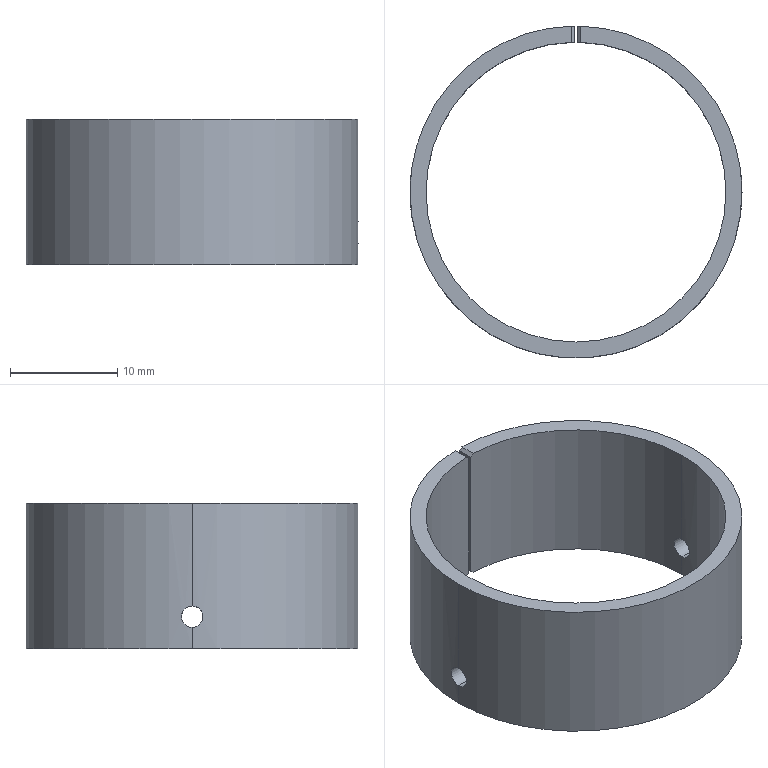Part | STEP file | TQ-DD-1105-THSHIELD1010_デフォルト | 1 solid | 18 faces | box 31 x 30.999 x 13.6 mm | volume 1876 mm3 | cylinder 10 | plane 8 | commonest cylinder face diameters 2 x4 28 x3 31 x3
STEP:
#1=CARTESIAN_POINT('',(-0.4352,15.494,0.));
#2=VERTEX_POINT('',#1);
#3=CARTESIAN_POINT('',(-15.5,0.,0.));
#4=VERTEX_POINT('',#3);
#5=CARTESIAN_POINT('',(0.,0.,0.));
#6=DIRECTION('',(0.,0.,1.));
#7=DIRECTION('',(1.,0.,0.));
#8=AXIS2_PLACEMENT_3D('',#5,#6,#7);
#9=CIRCLE('',#8,15.5);
#10=EDGE_CURVE('',#2,#4,#9,.T.);
#11=ORIENTED_EDGE('',*,*,#10,.T.);
#12=CARTESIAN_POINT('',(-15.5,0.,2.));
#13=VERTEX_POINT('',#12);
#14=CARTESIAN_POINT('',(-15.5,0.,6.8));
#15=DIRECTION('',(0.,0.,1.));
#16=VECTOR('',#15,1000.);
#17=LINE('',#14,#16);
#18=EDGE_CURVE('',#4,#13,#17,.T.);
#19=ORIENTED_EDGE('',*,*,#18,.T.);
#20=CARTESIAN_POINT('',(-15.5,0.,4.));
#21=VERTEX_POINT('',#20);
#22=CARTESIAN_POINT('',(-15.5,0.,2.));
#23=CARTESIAN_POINT('',(-15.5,0.1305,2.));
#24=CARTESIAN_POINT('',(-15.498,0.2615,2.026));
#25=CARTESIAN_POINT('',(-15.492,0.5036,2.126));
#26=CARTESIAN_POINT('',(-15.488,0.6138,2.2));
#27=CARTESIAN_POINT('',(-15.48,0.8004,2.386));
#28=CARTESIAN_POINT('',(-15.475,0.8738,2.496));
#29=CARTESIAN_POINT('',(-15.469,0.9741,2.739));
#30=CARTESIAN_POINT('',(-15.468,1.,2.869));
#31=CARTESIAN_POINT('',(-15.468,0.9999,3.133));
#32=CARTESIAN_POINT('',(-15.469,0.9738,3.263));
#33=CARTESIAN_POINT('',(-15.475,0.8732,3.505));
#34=CARTESIAN_POINT('',(-15.48,0.7989,3.615));
#35=CARTESIAN_POINT('',(-15.488,0.6143,3.8));
#36=CARTESIAN_POINT('',(-15.492,0.5027,3.874));
#37=CARTESIAN_POINT('',(-15.498,0.2621,3.974));
#38=CARTESIAN_POINT('',(-15.5,0.1305,4.));
#39=CARTESIAN_POINT('',(-15.5,0.,4.));
#40=B_SPLINE_CURVE_WITH_KNOTS('',3,(#22,#23,#24,#25,#26,#27,#28,#29,#30,#31,#32,#33,#34,#35,#36,#37,#38,#39),.UNSPECIFIED.,.F.,.F.,(4,2,2,2,2,2,2,2,4),(0.001564,0.001955,0.002346,0.002736,0.003127,0.003518,0.003909,0.0043,0.004691),.UNSPECIFIED.);
#41=EDGE_CURVE('',#13,#21,#40,.T.);
#42=ORIENTED_EDGE('',*,*,#41,.T.);
#43=CARTESIAN_POINT('',(-15.5,0.,13.6));
#44=VERTEX_POINT('',#43);
#45=CARTESIAN_POINT('',(-15.5,0.,6.8));
#46=DIRECTION('',(0.,0.,1.));
#47=VECTOR('',#46,1000.);
#48=LINE('',#45,#47);
#49=EDGE_CURVE('',#21,#44,#48,.T.);
#50=ORIENTED_EDGE('',*,*,#49,.T.);
#51=CARTESIAN_POINT('',(-0.4352,15.494,13.6));
#52=VERTEX_POINT('',#51);
#53=CARTESIAN_POINT('',(0.,0.,13.6));
#54=DIRECTION('',(0.,0.,-1.));
#55=DIRECTION('',(1.,0.,0.));
#56=AXIS2_PLACEMENT_3D('',#53,#54,#55);
#57=CIRCLE('',#56,15.5);
#58=EDGE_CURVE('',#44,#52,#57,.T.);
#59=ORIENTED_EDGE('',*,*,#58,.T.);
#60=CARTESIAN_POINT('',(-0.1353,15.499,13.3));
#61=VERTEX_POINT('',#60);
#62=CARTESIAN_POINT('',(-0.1353,15.499,13.3));
#63=CARTESIAN_POINT('',(-0.2353,15.499,13.4));
#64=CARTESIAN_POINT('',(-0.3353,15.497,13.5));
#65=CARTESIAN_POINT('',(-0.4352,15.494,13.6));
#66=(BOUNDED_CURVE()B_SPLINE_CURVE(3,(#62,#63,#64,#65),.UNSPECIFIED.,.F.,.F.)B_SPLINE_CURVE_WITH_KNOTS((4,4),(4.712,4.732),.UNSPECIFIED.)CURVE()GEOMETRIC_REPRESENTATION_ITEM()RATIONAL_B_SPLINE_CURVE((1.,1.,1.,1.))REPRESENTATION_ITEM(''));
#67=EDGE_CURVE('',#61,#52,#66,.T.);
#68=ORIENTED_EDGE('',*,*,#67,.F.);
#69=CARTESIAN_POINT('',(-0.1353,15.499,0.3));
#70=VERTEX_POINT('',#69);
#71=CARTESIAN_POINT('',(-0.1353,15.499,6.8));
#72=DIRECTION('',(0.,0.,-1.));
#73=VECTOR('',#72,1000.);
#74=LINE('',#71,#73);
#75=EDGE_CURVE('',#61,#70,#74,.T.);
#76=ORIENTED_EDGE('',*,*,#75,.T.);
#77=CARTESIAN_POINT('',(-0.1353,15.499,0.3));
#78=CARTESIAN_POINT('',(-0.2353,15.499,0.2));
#79=CARTESIAN_POINT('',(-0.3353,15.497,0.09999));
#80=CARTESIAN_POINT('',(-0.4352,15.494,0.));
#81=(BOUNDED_CURVE()B_SPLINE_CURVE(3,(#77,#78,#79,#80),.UNSPECIFIED.,.F.,.F.)B_SPLINE_CURVE_WITH_KNOTS((4,4),(1.571,1.59),.UNSPECIFIED.)CURVE()GEOMETRIC_REPRESENTATION_ITEM()RATIONAL_B_SPLINE_CURVE((1.,1.,1.,1.))REPRESENTATION_ITEM(''));
#82=EDGE_CURVE('',#70,#2,#81,.T.);
#83=ORIENTED_EDGE('',*,*,#82,.T.);
#84=EDGE_LOOP('',(#11,#19,#42,#50,#59,#68,#76,#83));
#85=FACE_OUTER_BOUND('',#84,.T.);
#86=CARTESIAN_POINT('',(0.,0.,6.8));
#87=DIRECTION('',(0.,0.,1.));
#88=DIRECTION('',(1.,0.,0.));
#89=AXIS2_PLACEMENT_3D('',#86,#87,#88);
#90=CYLINDRICAL_SURFACE('',#89,15.5);
#91=ADVANCED_FACE('',(#85),#90,.T.);
#92=ORIENTED_EDGE('',*,*,#18,.F.);
#93=CARTESIAN_POINT('',(15.5,0.,0.));
#94=VERTEX_POINT('',#93);
#95=CARTESIAN_POINT('',(0.,0.,0.));
#96=DIRECTION('',(0.,0.,1.));
#97=DIRECTION('',(1.,0.,0.));
#98=AXIS2_PLACEMENT_3D('',#95,#96,#97);
#99=CIRCLE('',#98,15.5);
#100=EDGE_CURVE('',#4,#94,#99,.T.);
#101=ORIENTED_EDGE('',*,*,#100,.T.);
#102=CARTESIAN_POINT('',(15.5,0.,2.));
#103=VERTEX_POINT('',#102);
#104=CARTESIAN_POINT('',(15.5,0.,6.8));
#105=DIRECTION('',(0.,0.,1.));
#106=VECTOR('',#105,1000.);
#107=LINE('',#104,#106);
#108=EDGE_CURVE('',#94,#103,#107,.T.);
#109=ORIENTED_EDGE('',*,*,#108,.T.);
#110=CARTESIAN_POINT('',(15.5,0.,4.));
#111=VERTEX_POINT('',#110);
#112=CARTESIAN_POINT('',(15.5,0.,2.));
#113=CARTESIAN_POINT('',(15.5,-0.1305,2.));
#114=CARTESIAN_POINT('',(15.498,-0.2615,2.026));
#115=CARTESIAN_POINT('',(15.492,-0.5036,2.126));
#116=CARTESIAN_POINT('',(15.488,-0.6137,2.2));
#117=CARTESIAN_POINT('',(15.48,-0.8004,2.386));
#118=CARTESIAN_POINT('',(15.475,-0.8738,2.496));
#119=CARTESIAN_POINT('',(15.469,-0.9741,2.739));
#120=CARTESIAN_POINT('',(15.468,-1.,2.869));
#121=CARTESIAN_POINT('',(15.468,-0.9999,3.133));
#122=CARTESIAN_POINT('',(15.469,-0.9738,3.263));
#123=CARTESIAN_POINT('',(15.475,-0.8732,3.505));
#124=CARTESIAN_POINT('',(15.48,-0.7989,3.615));
#125=CARTESIAN_POINT('',(15.488,-0.6143,3.8));
#126=CARTESIAN_POINT('',(15.492,-0.5027,3.874));
#127=CARTESIAN_POINT('',(15.498,-0.2621,3.974));
#128=CARTESIAN_POINT('',(15.5,-0.1305,4.));
#129=CARTESIAN_POINT('',(15.5,0.,4.));
#130=B_SPLINE_CURVE_WITH_KNOTS('',3,(#112,#113,#114,#115,#116,#117,#118,#119,#120,#121,#122,#123,#124,#125,#126,#127,#128,#129),.UNSPECIFIED.,.F.,.F.,(4,2,2,2,2,2,2,2,4),(0.004691,0.005081,0.005472,0.005863,0.006254,0.006645,0.007036,0.007426,0.007817),.UNSPECIFIED.);
#131=EDGE_CURVE('',#103,#111,#130,.T.);
#132=ORIENTED_EDGE('',*,*,#131,.T.);
#133=CARTESIAN_POINT('',(15.5,0.,13.6));
#134=VERTEX_POINT('',#133);
#135=CARTESIAN_POINT('',(15.5,0.,6.8));
#136=DIRECTION('',(0.,0.,1.));
#137=VECTOR('',#136,1000.);
#138=LINE('',#135,#137);
#139=EDGE_CURVE('',#111,#134,#138,.T.);
#140=ORIENTED_EDGE('',*,*,#139,.T.);
#141=CARTESIAN_POINT('',(0.,0.,13.6));
#142=DIRECTION('',(0.,0.,-1.));
#143=DIRECTION('',(1.,0.,0.));
#144=AXIS2_PLACEMENT_3D('',#141,#142,#143);
#145=CIRCLE('',#144,15.5);
#146=EDGE_CURVE('',#134,#44,#145,.T.);
#147=ORIENTED_EDGE('',*,*,#146,.T.);
#148=ORIENTED_EDGE('',*,*,#49,.F.);
#149=CARTESIAN_POINT('',(-15.5,0.,4.));
#150=CARTESIAN_POINT('',(-15.5,-0.1305,4.));
#151=CARTESIAN_POINT('',(-15.498,-0.2615,3.974));
#152=CARTESIAN_POINT('',(-15.492,-0.5036,3.874));
#153=CARTESIAN_POINT('',(-15.488,-0.6137,3.8));
#154=CARTESIAN_POINT('',(-15.48,-0.8004,3.614));
#155=CARTESIAN_POINT('',(-15.475,-0.8738,3.504));
#156=CARTESIAN_POINT('',(-15.469,-0.9741,3.261));
#157=CARTESIAN_POINT('',(-15.468,-1.,3.131));
#158=CARTESIAN_POINT('',(-15.468,-0.9999,2.867));
#159=CARTESIAN_POINT('',(-15.469,-0.9738,2.737));
#160=CARTESIAN_POINT('',(-15.475,-0.8732,2.495));
#161=CARTESIAN_POINT('',(-15.48,-0.7989,2.385));
#162=CARTESIAN_POINT('',(-15.488,-0.6143,2.2));
#163=CARTESIAN_POINT('',(-15.492,-0.5027,2.126));
#164=CARTESIAN_POINT('',(-15.498,-0.2621,2.026));
#165=CARTESIAN_POINT('',(-15.5,-0.1305,2.));
#166=CARTESIAN_POINT('',(-15.5,0.,2.));
#167=B_SPLINE_CURVE_WITH_KNOTS('',3,(#149,#150,#151,#152,#153,#154,#155,#156,#157,#158,#159,#160,#161,#162,#163,#164,#165,#166),.UNSPECIFIED.,.F.,.F.,(4,2,2,2,2,2,2,2,4),(0.004691,0.005081,0.005472,0.005863,0.006254,0.006645,0.007036,0.007426,0.007817),.UNSPECIFIED.);
#168=EDGE_CURVE('',#21,#13,#167,.T.);
#169=ORIENTED_EDGE('',*,*,#168,.T.);
#170=EDGE_LOOP('',(#92,#101,#109,#132,#140,#147,#148,#169));
#171=FACE_OUTER_BOUND('',#170,.T.);
#172=CARTESIAN_POINT('',(0.,0.,6.8));
#173=DIRECTION('',(0.,0.,1.));
#174=DIRECTION('',(1.,0.,0.));
#175=AXIS2_PLACEMENT_3D('',#172,#173,#174);
#176=CYLINDRICAL_SURFACE('',#175,15.5);
#177=ADVANCED_FACE('',(#171),#176,.T.);
#178=CARTESIAN_POINT('',(14.,0.,4.));
#179=VERTEX_POINT('',#178);
#180=CARTESIAN_POINT('',(14.,0.,2.));
#181=VERTEX_POINT('',#180);
#182=CARTESIAN_POINT('',(14.,0.,4.));
#183=CARTESIAN_POINT('',(14.,-0.1305,4.));
#184=CARTESIAN_POINT('',(13.998,-0.2615,3.974));
#185=CARTESIAN_POINT('',(13.991,-0.5037,3.874));
#186=CARTESIAN_POINT('',(13.987,-0.6138,3.8));
#187=CARTESIAN_POINT('',(13.977,-0.8005,3.614));
#188=CARTESIAN_POINT('',(13.973,-0.8738,3.504));
#189=CARTESIAN_POINT('',(13.966,-0.9741,3.261));
#190=CARTESIAN_POINT('',(13.964,-1.,3.131));
#191=CARTESIAN_POINT('',(13.964,-0.9999,2.867));
#192=CARTESIAN_POINT('',(13.966,-0.9738,2.737));
#193=CARTESIAN_POINT('',(13.973,-0.8732,2.495));
#194=CARTESIAN_POINT('',(13.977,-0.7989,2.385));
#195=CARTESIAN_POINT('',(13.987,-0.6143,2.2));
#196=CARTESIAN_POINT('',(13.991,-0.5028,2.126));
#197=CARTESIAN_POINT('',(13.998,-0.2621,2.026));
#198=CARTESIAN_POINT('',(14.,-0.1305,2.));
#199=CARTESIAN_POINT('',(14.,0.,2.));
#200=B_SPLINE_CURVE_WITH_KNOTS('',3,(#182,#183,#184,#185,#186,#187,#188,#189,#190,#191,#192,#193,#194,#195,#196,#197,#198,#199),.UNSPECIFIED.,.F.,.F.,(4,2,2,2,2,2,2,2,4),(0.004691,0.005082,0.005473,0.005863,0.006254,0.006645,0.007036,0.007427,0.007818),.UNSPECIFIED.);
#201=EDGE_CURVE('',#179,#181,#200,.T.);
#202=ORIENTED_EDGE('',*,*,#201,.F.);
#203=CARTESIAN_POINT('',(0.,0.,4.));
#204=DIRECTION('',(1.,0.,0.));
#205=VECTOR('',#204,1000.);
#206=LINE('',#203,#205);
#207=EDGE_CURVE('',#179,#111,#206,.T.);
#208=ORIENTED_EDGE('',*,*,#207,.T.);
#209=ORIENTED_EDGE('',*,*,#131,.F.);
#210=CARTESIAN_POINT('',(0.,0.,2.));
#211=DIRECTION('',(1.,0.,0.));
#212=VECTOR('',#211,1000.);
#213=LINE('',#210,#212);
#214=EDGE_CURVE('',#181,#103,#213,.T.);
#215=ORIENTED_EDGE('',*,*,#214,.F.);
#216=EDGE_LOOP('',(#202,#208,#209,#215));
#217=FACE_OUTER_BOUND('',#216,.T.);
#218=CARTESIAN_POINT('',(0.,0.,3.));
#219=DIRECTION('',(1.,0.,0.));
#220=DIRECTION('',(0.,0.,-1.));
#221=AXIS2_PLACEMENT_3D('',#218,#219,#220);
#222=CYLINDRICAL_SURFACE('',#221,1.);
#223=ADVANCED_FACE('',(#217),#222,.F.);
#224=ORIENTED_EDGE('',*,*,#168,.F.);
#225=CARTESIAN_POINT('',(-14.,0.,4.));
#226=VERTEX_POINT('',#225);
#227=CARTESIAN_POINT('',(0.,0.,4.));
#228=DIRECTION('',(1.,0.,0.));
#229=VECTOR('',#228,1000.);
#230=LINE('',#227,#229);
#231=EDGE_CURVE('',#21,#226,#230,.T.);
#232=ORIENTED_EDGE('',*,*,#231,.T.);
#233=CARTESIAN_POINT('',(-14.,0.,2.));
#234=VERTEX_POINT('',#233);
#235=CARTESIAN_POINT('',(-14.,0.,2.));
#236=CARTESIAN_POINT('',(-14.,-0.1305,2.));
#237=CARTESIAN_POINT('',(-13.998,-0.2615,2.026));
#238=CARTESIAN_POINT('',(-13.991,-0.5037,2.126));
#239=CARTESIAN_POINT('',(-13.987,-0.6138,2.2));
#240=CARTESIAN_POINT('',(-13.977,-0.8005,2.386));
#241=CARTESIAN_POINT('',(-13.973,-0.8738,2.496));
#242=CARTESIAN_POINT('',(-13.966,-0.9741,2.739));
#243=CARTESIAN_POINT('',(-13.964,-1.,2.869));
#244=CARTESIAN_POINT('',(-13.964,-0.9999,3.133));
#245=CARTESIAN_POINT('',(-13.966,-0.9738,3.263));
#246=CARTESIAN_POINT('',(-13.973,-0.8732,3.505));
#247=CARTESIAN_POINT('',(-13.977,-0.7989,3.615));
#248=CARTESIAN_POINT('',(-13.987,-0.6143,3.8));
#249=CARTESIAN_POINT('',(-13.991,-0.5028,3.874));
#250=CARTESIAN_POINT('',(-13.998,-0.2621,3.974));
#251=CARTESIAN_POINT('',(-14.,-0.1305,4.));
#252=CARTESIAN_POINT('',(-14.,0.,4.));
#253=B_SPLINE_CURVE_WITH_KNOTS('',3,(#235,#236,#237,#238,#239,#240,#241,#242,#243,#244,#245,#246,#247,#248,#249,#250,#251,#252),.UNSPECIFIED.,.F.,.F.,(4,2,2,2,2,2,2,2,4),(0.004691,0.005082,0.005473,0.005863,0.006254,0.006645,0.007036,0.007427,0.007818),.UNSPECIFIED.);
#254=EDGE_CURVE('',#234,#226,#253,.T.);
#255=ORIENTED_EDGE('',*,*,#254,.F.);
#256=CARTESIAN_POINT('',(0.,0.,2.));
#257=DIRECTION('',(1.,0.,0.));
#258=VECTOR('',#257,1000.);
#259=LINE('',#256,#258);
#260=EDGE_CURVE('',#13,#234,#259,.T.);
#261=ORIENTED_EDGE('',*,*,#260,.F.);
#262=EDGE_LOOP('',(#224,#232,#255,#261));
#263=FACE_OUTER_BOUND('',#262,.T.);
#264=CARTESIAN_POINT('',(0.,0.,3.));
#265=DIRECTION('',(1.,0.,0.));
#266=DIRECTION('',(0.,0.,-1.));
#267=AXIS2_PLACEMENT_3D('',#264,#265,#266);
#268=CYLINDRICAL_SURFACE('',#267,1.);
#269=ADVANCED_FACE('',(#263),#268,.F.);
#270=CARTESIAN_POINT('',(14.,0.,0.));
#271=VERTEX_POINT('',#270);
#272=CARTESIAN_POINT('',(-14.,0.,0.));
#273=VERTEX_POINT('',#272);
#274=CARTESIAN_POINT('',(0.,0.,0.));
#275=DIRECTION('',(0.,0.,-1.));
#276=DIRECTION('',(1.,0.,0.));
#277=AXIS2_PLACEMENT_3D('',#274,#275,#276);
#278=CIRCLE('',#277,14.);
#279=EDGE_CURVE('',#271,#273,#278,.T.);
#280=ORIENTED_EDGE('',*,*,#279,.T.);
#281=CARTESIAN_POINT('',(-14.,0.,6.8));
#282=DIRECTION('',(0.,0.,1.));
#283=VECTOR('',#282,1000.);
#284=LINE('',#281,#283);
#285=EDGE_CURVE('',#273,#234,#284,.T.);
#286=ORIENTED_EDGE('',*,*,#285,.T.);
#287=ORIENTED_EDGE('',*,*,#254,.T.);
#288=CARTESIAN_POINT('',(-14.,0.,13.6));
#289=VERTEX_POINT('',#288);
#290=CARTESIAN_POINT('',(-14.,0.,6.8));
#291=DIRECTION('',(0.,0.,1.));
#292=VECTOR('',#291,1000.);
#293=LINE('',#290,#292);
#294=EDGE_CURVE('',#226,#289,#293,.T.);
#295=ORIENTED_EDGE('',*,*,#294,.T.);
#296=CARTESIAN_POINT('',(14.,0.,13.6));
#297=VERTEX_POINT('',#296);
#298=CARTESIAN_POINT('',(0.,0.,13.6));
#299=DIRECTION('',(0.,0.,-1.));
#300=DIRECTION('',(1.,0.,0.));
#301=AXIS2_PLACEMENT_3D('',#298,#299,#300);
#302=CIRCLE('',#301,14.);
#303=EDGE_CURVE('',#297,#289,#302,.T.);
#304=ORIENTED_EDGE('',*,*,#303,.F.);
#305=CARTESIAN_POINT('',(14.,0.,6.8));
#306=DIRECTION('',(0.,0.,1.));
#307=VECTOR('',#306,1000.);
#308=LINE('',#305,#307);
#309=EDGE_CURVE('',#179,#297,#308,.T.);
#310=ORIENTED_EDGE('',*,*,#309,.F.);
#311=ORIENTED_EDGE('',*,*,#201,.T.);
#312=CARTESIAN_POINT('',(14.,0.,6.8));
#313=DIRECTION('',(0.,0.,1.));
#314=VECTOR('',#313,1000.);
#315=LINE('',#312,#314);
#316=EDGE_CURVE('',#271,#181,#315,.T.);
#317=ORIENTED_EDGE('',*,*,#316,.F.);
#318=EDGE_LOOP('',(#280,#286,#287,#295,#304,#310,#311,#317));
#319=FACE_OUTER_BOUND('',#318,.T.);
#320=CARTESIAN_POINT('',(0.,0.,6.8));
#321=DIRECTION('',(0.,0.,1.));
#322=DIRECTION('',(1.,0.,0.));
#323=AXIS2_PLACEMENT_3D('',#320,#321,#322);
#324=CYLINDRICAL_SURFACE('',#323,14.);
#325=ADVANCED_FACE('',(#319),#324,.F.);
#326=CARTESIAN_POINT('',(0.4221,13.994,0.));
#327=VERTEX_POINT('',#326);
#328=CARTESIAN_POINT('',(0.,0.,0.));
#329=DIRECTION('',(0.,0.,-1.));
#330=DIRECTION('',(1.,0.,0.));
#331=AXIS2_PLACEMENT_3D('',#328,#329,#330);
#332=CIRCLE('',#331,14.);
#333=EDGE_CURVE('',#327,#271,#332,.T.);
#334=ORIENTED_EDGE('',*,*,#333,.T.);
#335=ORIENTED_EDGE('',*,*,#316,.T.);
#336=CARTESIAN_POINT('',(14.,0.,2.));
#337=CARTESIAN_POINT('',(14.,0.1305,2.));
#338=CARTESIAN_POINT('',(13.998,0.2615,2.026));
#339=CARTESIAN_POINT('',(13.991,0.5037,2.126));
#340=CARTESIAN_POINT('',(13.987,0.6138,2.2));
#341=CARTESIAN_POINT('',(13.977,0.8005,2.386));
#342=CARTESIAN_POINT('',(13.973,0.8738,2.496));
#343=CARTESIAN_POINT('',(13.966,0.9741,2.739));
#344=CARTESIAN_POINT('',(13.964,1.,2.869));
#345=CARTESIAN_POINT('',(13.964,0.9999,3.133));
#346=CARTESIAN_POINT('',(13.966,0.9738,3.263));
#347=CARTESIAN_POINT('',(13.973,0.8732,3.505));
#348=CARTESIAN_POINT('',(13.977,0.7989,3.615));
#349=CARTESIAN_POINT('',(13.987,0.6143,3.8));
#350=CARTESIAN_POINT('',(13.991,0.5028,3.874));
#351=CARTESIAN_POINT('',(13.998,0.2621,3.974));
#352=CARTESIAN_POINT('',(14.,0.1305,4.));
#353=CARTESIAN_POINT('',(14.,0.,4.));
#354=B_SPLINE_CURVE_WITH_KNOTS('',3,(#336,#337,#338,#339,#340,#341,#342,#343,#344,#345,#346,#347,#348,#349,#350,#351,#352,#353),.UNSPECIFIED.,.F.,.F.,(4,2,2,2,2,2,2,2,4),(0.001564,0.001955,0.002346,0.002737,0.003127,0.003518,0.003909,0.0043,0.004691),.UNSPECIFIED.);
#355=EDGE_CURVE('',#181,#179,#354,.T.);
#356=ORIENTED_EDGE('',*,*,#355,.T.);
#357=ORIENTED_EDGE('',*,*,#309,.T.);
#358=CARTESIAN_POINT('',(0.4221,13.994,13.6));
#359=VERTEX_POINT('',#358);
#360=CARTESIAN_POINT('',(0.,0.,13.6));
#361=DIRECTION('',(0.,0.,-1.));
#362=DIRECTION('',(1.,0.,0.));
#363=AXIS2_PLACEMENT_3D('',#360,#361,#362);
#364=CIRCLE('',#363,14.);
#365=EDGE_CURVE('',#359,#297,#364,.T.);
#366=ORIENTED_EDGE('',*,*,#365,.F.);
#367=CARTESIAN_POINT('',(0.1222,13.999,13.3));
#368=VERTEX_POINT('',#367);
#369=CARTESIAN_POINT('',(0.1222,13.999,13.3));
#370=CARTESIAN_POINT('',(0.2222,13.999,13.4));
#371=CARTESIAN_POINT('',(0.3222,13.997,13.5));
#372=CARTESIAN_POINT('',(0.4221,13.994,13.6));
#373=(BOUNDED_CURVE()B_SPLINE_CURVE(3,(#369,#370,#371,#372),.UNSPECIFIED.,.F.,.F.)B_SPLINE_CURVE_WITH_KNOTS((4,4),(4.712,4.734),.UNSPECIFIED.)CURVE()GEOMETRIC_REPRESENTATION_ITEM()RATIONAL_B_SPLINE_CURVE((1.,1.,1.,1.))REPRESENTATION_ITEM(''));
#374=EDGE_CURVE('',#368,#359,#373,.T.);
#375=ORIENTED_EDGE('',*,*,#374,.F.);
#376=CARTESIAN_POINT('',(0.1222,13.999,0.3));
#377=VERTEX_POINT('',#376);
#378=CARTESIAN_POINT('',(0.1222,13.999,0.));
#379=DIRECTION('',(0.,0.,1.));
#380=VECTOR('',#379,1000.);
#381=LINE('',#378,#380);
#382=EDGE_CURVE('',#377,#368,#381,.T.);
#383=ORIENTED_EDGE('',*,*,#382,.F.);
#384=CARTESIAN_POINT('',(0.4221,13.994,0.));
#385=CARTESIAN_POINT('',(0.3222,13.997,0.09999));
#386=CARTESIAN_POINT('',(0.2222,13.999,0.2));
#387=CARTESIAN_POINT('',(0.1222,13.999,0.3));
#388=(BOUNDED_CURVE()B_SPLINE_CURVE(3,(#384,#385,#386,#387),.UNSPECIFIED.,.F.,.F.)B_SPLINE_CURVE_WITH_KNOTS((4,4),(4.691,4.712),.UNSPECIFIED.)CURVE()GEOMETRIC_REPRESENTATION_ITEM()RATIONAL_B_SPLINE_CURVE((1.,1.,1.,1.))REPRESENTATION_ITEM(''));
#389=EDGE_CURVE('',#327,#377,#388,.T.);
#390=ORIENTED_EDGE('',*,*,#389,.F.);
#391=EDGE_LOOP('',(#334,#335,#356,#357,#366,#375,#383,#390));
#392=FACE_OUTER_BOUND('',#391,.T.);
#393=CARTESIAN_POINT('',(0.,0.,6.8));
#394=DIRECTION('',(0.,0.,1.));
#395=DIRECTION('',(1.,0.,0.));
#396=AXIS2_PLACEMENT_3D('',#393,#394,#395);
#397=CYLINDRICAL_SURFACE('',#396,14.);
#398=ADVANCED_FACE('',(#392),#397,.F.);
#399=ORIENTED_EDGE('',*,*,#108,.F.);
#400=CARTESIAN_POINT('',(0.4352,15.494,0.));
#401=VERTEX_POINT('',#400);
#402=CARTESIAN_POINT('',(0.,0.,0.));
#403=DIRECTION('',(0.,0.,1.));
#404=DIRECTION('',(1.,0.,0.));
#405=AXIS2_PLACEMENT_3D('',#402,#403,#404);
#406=CIRCLE('',#405,15.5);
#407=EDGE_CURVE('',#94,#401,#406,.T.);
#408=ORIENTED_EDGE('',*,*,#407,.T.);
#409=CARTESIAN_POINT('',(0.1353,15.499,0.3));
#410=VERTEX_POINT('',#409);
#411=CARTESIAN_POINT('',(0.1353,15.499,0.3));
#412=CARTESIAN_POINT('',(0.2353,15.499,0.2));
#413=CARTESIAN_POINT('',(0.3353,15.497,0.09999));
#414=CARTESIAN_POINT('',(0.4352,15.494,0.));
#415=(BOUNDED_CURVE()B_SPLINE_CURVE(3,(#411,#412,#413,#414),.UNSPECIFIED.,.F.,.F.)B_SPLINE_CURVE_WITH_KNOTS((4,4),(1.571,1.59),.UNSPECIFIED.)CURVE()GEOMETRIC_REPRESENTATION_ITEM()RATIONAL_B_SPLINE_CURVE((1.,1.,1.,1.))REPRESENTATION_ITEM(''));
#416=EDGE_CURVE('',#410,#401,#415,.T.);
#417=ORIENTED_EDGE('',*,*,#416,.F.);
#418=CARTESIAN_POINT('',(0.1353,15.499,13.3));
#419=VERTEX_POINT('',#418);
#420=CARTESIAN_POINT('',(0.1353,15.499,6.8));
#421=DIRECTION('',(0.,0.,1.));
#422=VECTOR('',#421,1000.);
#423=LINE('',#420,#422);
#424=EDGE_CURVE('',#410,#419,#423,.T.);
#425=ORIENTED_EDGE('',*,*,#424,.T.);
#426=CARTESIAN_POINT('',(0.4352,15.494,13.6));
#427=VERTEX_POINT('',#426);
#428=CARTESIAN_POINT('',(0.1353,15.499,13.3));
#429=CARTESIAN_POINT('',(0.2353,15.499,13.4));
#430=CARTESIAN_POINT('',(0.3353,15.497,13.5));
#431=CARTESIAN_POINT('',(0.4352,15.494,13.6));
#432=(BOUNDED_CURVE()B_SPLINE_CURVE(3,(#428,#429,#430,#431),.UNSPECIFIED.,.F.,.F.)B_SPLINE_CURVE_WITH_KNOTS((4,4),(4.712,4.732),.UNSPECIFIED.)CURVE()GEOMETRIC_REPRESENTATION_ITEM()RATIONAL_B_SPLINE_CURVE((1.,1.,1.,1.))REPRESENTATION_ITEM(''));
#433=EDGE_CURVE('',#419,#427,#432,.T.);
#434=ORIENTED_EDGE('',*,*,#433,.T.);
#435=CARTESIAN_POINT('',(0.,0.,13.6));
#436=DIRECTION('',(0.,0.,-1.));
#437=DIRECTION('',(1.,0.,0.));
#438=AXIS2_PLACEMENT_3D('',#435,#436,#437);
#439=CIRCLE('',#438,15.5);
#440=EDGE_CURVE('',#427,#134,#439,.T.);
#441=ORIENTED_EDGE('',*,*,#440,.T.);
#442=ORIENTED_EDGE('',*,*,#139,.F.);
#443=CARTESIAN_POINT('',(15.5,0.,4.));
#444=CARTESIAN_POINT('',(15.5,0.1305,4.));
#445=CARTESIAN_POINT('',(15.498,0.2615,3.974));
#446=CARTESIAN_POINT('',(15.492,0.5036,3.874));
#447=CARTESIAN_POINT('',(15.488,0.6138,3.8));
#448=CARTESIAN_POINT('',(15.48,0.8004,3.614));
#449=CARTESIAN_POINT('',(15.475,0.8738,3.504));
#450=CARTESIAN_POINT('',(15.469,0.9741,3.261));
#451=CARTESIAN_POINT('',(15.468,1.,3.131));
#452=CARTESIAN_POINT('',(15.468,0.9999,2.867));
#453=CARTESIAN_POINT('',(15.469,0.9738,2.737));
#454=CARTESIAN_POINT('',(15.475,0.8732,2.495));
#455=CARTESIAN_POINT('',(15.48,0.7989,2.385));
#456=CARTESIAN_POINT('',(15.488,0.6143,2.2));
#457=CARTESIAN_POINT('',(15.492,0.5027,2.126));
#458=CARTESIAN_POINT('',(15.498,0.2621,2.026));
#459=CARTESIAN_POINT('',(15.5,0.1305,2.));
#460=CARTESIAN_POINT('',(15.5,0.,2.));
#461=B_SPLINE_CURVE_WITH_KNOTS('',3,(#443,#444,#445,#446,#447,#448,#449,#450,#451,#452,#453,#454,#455,#456,#457,#458,#459,#460),.UNSPECIFIED.,.F.,.F.,(4,2,2,2,2,2,2,2,4),(0.001564,0.001955,0.002346,0.002736,0.003127,0.003518,0.003909,0.0043,0.004691),.UNSPECIFIED.);
#462=EDGE_CURVE('',#111,#103,#461,.T.);
#463=ORIENTED_EDGE('',*,*,#462,.T.);
#464=EDGE_LOOP('',(#399,#408,#417,#425,#434,#441,#442,#463));
#465=FACE_OUTER_BOUND('',#464,.T.);
#466=CARTESIAN_POINT('',(0.,0.,6.8));
#467=DIRECTION('',(0.,0.,1.));
#468=DIRECTION('',(1.,0.,0.));
#469=AXIS2_PLACEMENT_3D('',#466,#467,#468);
#470=CYLINDRICAL_SURFACE('',#469,15.5);
#471=ADVANCED_FACE('',(#465),#470,.T.);
#472=ORIENTED_EDGE('',*,*,#207,.F.);
#473=ORIENTED_EDGE('',*,*,#355,.F.);
#474=ORIENTED_EDGE('',*,*,#214,.T.);
#475=ORIENTED_EDGE('',*,*,#462,.F.);
#476=EDGE_LOOP('',(#472,#473,#474,#475));
#477=FACE_OUTER_BOUND('',#476,.T.);
#478=CARTESIAN_POINT('',(0.,0.,3.));
#479=DIRECTION('',(1.,0.,0.));
#480=DIRECTION('',(0.,0.,-1.));
#481=AXIS2_PLACEMENT_3D('',#478,#479,#480);
#482=CYLINDRICAL_SURFACE('',#481,1.);
#483=ADVANCED_FACE('',(#477),#482,.F.);
#484=ORIENTED_EDGE('',*,*,#231,.F.);
#485=ORIENTED_EDGE('',*,*,#41,.F.);
#486=ORIENTED_EDGE('',*,*,#260,.T.);
#487=CARTESIAN_POINT('',(-14.,0.,4.));
#488=CARTESIAN_POINT('',(-14.,0.1305,4.));
#489=CARTESIAN_POINT('',(-13.998,0.2615,3.974));
#490=CARTESIAN_POINT('',(-13.991,0.5037,3.874));
#491=CARTESIAN_POINT('',(-13.987,0.6138,3.8));
#492=CARTESIAN_POINT('',(-13.977,0.8005,3.614));
#493=CARTESIAN_POINT('',(-13.973,0.8738,3.504));
#494=CARTESIAN_POINT('',(-13.966,0.9741,3.261));
#495=CARTESIAN_POINT('',(-13.964,1.,3.131));
#496=CARTESIAN_POINT('',(-13.964,0.9999,2.867));
#497=CARTESIAN_POINT('',(-13.966,0.9738,2.737));
#498=CARTESIAN_POINT('',(-13.973,0.8732,2.495));
#499=CARTESIAN_POINT('',(-13.977,0.7989,2.385));
#500=CARTESIAN_POINT('',(-13.987,0.6143,2.2));
#501=CARTESIAN_POINT('',(-13.991,0.5028,2.126));
#502=CARTESIAN_POINT('',(-13.998,0.2621,2.026));
#503=CARTESIAN_POINT('',(-14.,0.1305,2.));
#504=CARTESIAN_POINT('',(-14.,0.,2.));
#505=B_SPLINE_CURVE_WITH_KNOTS('',3,(#487,#488,#489,#490,#491,#492,#493,#494,#495,#496,#497,#498,#499,#500,#501,#502,#503,#504),.UNSPECIFIED.,.F.,.F.,(4,2,2,2,2,2,2,2,4),(0.001564,0.001955,0.002346,0.002737,0.003127,0.003518,0.003909,0.0043,0.004691),.UNSPECIFIED.);
#506=EDGE_CURVE('',#226,#234,#505,.T.);
#507=ORIENTED_EDGE('',*,*,#506,.F.);
#508=EDGE_LOOP('',(#484,#485,#486,#507));
#509=FACE_OUTER_BOUND('',#508,.T.);
#510=CARTESIAN_POINT('',(0.,0.,3.));
#511=DIRECTION('',(1.,0.,0.));
#512=DIRECTION('',(0.,0.,-1.));
#513=AXIS2_PLACEMENT_3D('',#510,#511,#512);
#514=CYLINDRICAL_SURFACE('',#513,1.);
#515=ADVANCED_FACE('',(#509),#514,.F.);
#516=ORIENTED_EDGE('',*,*,#10,.F.);
#517=CARTESIAN_POINT('',(-0.4221,13.994,0.));
#518=VERTEX_POINT('',#517);
#519=CARTESIAN_POINT('',(-0.4221,13.994,0.));
#520=DIRECTION('',(-0.008727,1.,0.));
#521=VECTOR('',#520,1000.);
#522=LINE('',#519,#521);
#523=EDGE_CURVE('',#518,#2,#522,.T.);
#524=ORIENTED_EDGE('',*,*,#523,.F.);
#525=CARTESIAN_POINT('',(0.,0.,0.));
#526=DIRECTION('',(0.,0.,-1.));
#527=DIRECTION('',(1.,0.,0.));
#528=AXIS2_PLACEMENT_3D('',#525,#526,#527);
#529=CIRCLE('',#528,14.);
#530=EDGE_CURVE('',#273,#518,#529,.T.);
#531=ORIENTED_EDGE('',*,*,#530,.F.);
#532=ORIENTED_EDGE('',*,*,#279,.F.);
#533=ORIENTED_EDGE('',*,*,#333,.F.);
#534=CARTESIAN_POINT('',(0.4352,15.494,0.));
#535=DIRECTION('',(-0.008727,-1.,0.));
#536=VECTOR('',#535,1000.);
#537=LINE('',#534,#536);
#538=EDGE_CURVE('',#401,#327,#537,.T.);
#539=ORIENTED_EDGE('',*,*,#538,.F.);
#540=ORIENTED_EDGE('',*,*,#407,.F.);
#541=ORIENTED_EDGE('',*,*,#100,.F.);
#542=EDGE_LOOP('',(#516,#524,#531,#532,#533,#539,#540,#541));
#543=FACE_OUTER_BOUND('',#542,.T.);
#544=CARTESIAN_POINT('',(0.,0.,0.));
#545=DIRECTION('',(0.,0.,1.));
#546=DIRECTION('',(1.,0.,0.));
#547=AXIS2_PLACEMENT_3D('',#544,#545,#546);
#548=PLANE('',#547);
#549=ADVANCED_FACE('',(#543),#548,.F.);
#550=ORIENTED_EDGE('',*,*,#75,.F.);
#551=CARTESIAN_POINT('',(-0.1222,13.999,13.3));
#552=VERTEX_POINT('',#551);
#553=CARTESIAN_POINT('',(-0.1353,15.499,13.3));
#554=DIRECTION('',(-0.008727,1.,0.));
#555=VECTOR('',#554,1000.);
#556=LINE('',#553,#555);
#557=EDGE_CURVE('',#552,#61,#556,.T.);
#558=ORIENTED_EDGE('',*,*,#557,.F.);
#559=CARTESIAN_POINT('',(-0.1222,13.999,0.3));
#560=VERTEX_POINT('',#559);
#561=CARTESIAN_POINT('',(-0.1222,13.999,0.));
#562=DIRECTION('',(0.,0.,1.));
#563=VECTOR('',#562,1000.);
#564=LINE('',#561,#563);
#565=EDGE_CURVE('',#560,#552,#564,.T.);
#566=ORIENTED_EDGE('',*,*,#565,.F.);
#567=CARTESIAN_POINT('',(-0.1353,15.499,0.3));
#568=DIRECTION('',(0.008727,-1.,0.));
#569=VECTOR('',#568,1000.);
#570=LINE('',#567,#569);
#571=EDGE_CURVE('',#70,#560,#570,.T.);
#572=ORIENTED_EDGE('',*,*,#571,.F.);
#573=EDGE_LOOP('',(#550,#558,#566,#572));
#574=FACE_OUTER_BOUND('',#573,.T.);
#575=CARTESIAN_POINT('',(-0.1353,15.499,0.));
#576=DIRECTION('',(-1.,-0.008727,0.));
#577=DIRECTION('',(0.008727,-1.,0.));
#578=AXIS2_PLACEMENT_3D('',#575,#576,#577);
#579=PLANE('',#578);
#580=ADVANCED_FACE('',(#574),#579,.F.);
#581=ORIENTED_EDGE('',*,*,#440,.F.);
#582=CARTESIAN_POINT('',(0.4352,15.494,13.6));
#583=DIRECTION('',(-0.008727,-1.,0.));
#584=VECTOR('',#583,1000.);
#585=LINE('',#582,#584);
#586=EDGE_CURVE('',#427,#359,#585,.T.);
#587=ORIENTED_EDGE('',*,*,#586,.T.);
#588=ORIENTED_EDGE('',*,*,#365,.T.);
#589=ORIENTED_EDGE('',*,*,#303,.T.);
#590=CARTESIAN_POINT('',(-0.4221,13.994,13.6));
#591=VERTEX_POINT('',#590);
#592=CARTESIAN_POINT('',(0.,0.,13.6));
#593=DIRECTION('',(0.,0.,-1.));
#594=DIRECTION('',(1.,0.,0.));
#595=AXIS2_PLACEMENT_3D('',#592,#593,#594);
#596=CIRCLE('',#595,14.);
#597=EDGE_CURVE('',#289,#591,#596,.T.);
#598=ORIENTED_EDGE('',*,*,#597,.T.);
#599=CARTESIAN_POINT('',(-0.4221,13.994,13.6));
#600=DIRECTION('',(-0.008727,1.,0.));
#601=VECTOR('',#600,1000.);
#602=LINE('',#599,#601);
#603=EDGE_CURVE('',#591,#52,#602,.T.);
#604=ORIENTED_EDGE('',*,*,#603,.T.);
#605=ORIENTED_EDGE('',*,*,#58,.F.);
#606=ORIENTED_EDGE('',*,*,#146,.F.);
#607=EDGE_LOOP('',(#581,#587,#588,#589,#598,#604,#605,#606));
#608=FACE_OUTER_BOUND('',#607,.T.);
#609=CARTESIAN_POINT('',(0.,0.,13.6));
#610=DIRECTION('',(0.,0.,1.));
#611=DIRECTION('',(1.,0.,0.));
#612=AXIS2_PLACEMENT_3D('',#609,#610,#611);
#613=PLANE('',#612);
#614=ADVANCED_FACE('',(#608),#613,.T.);
#615=ORIENTED_EDGE('',*,*,#424,.F.);
#616=CARTESIAN_POINT('',(0.1353,15.499,0.3));
#617=DIRECTION('',(-0.008727,-1.,0.));
#618=VECTOR('',#617,1000.);
#619=LINE('',#616,#618);
#620=EDGE_CURVE('',#410,#377,#619,.T.);
#621=ORIENTED_EDGE('',*,*,#620,.T.);
#622=ORIENTED_EDGE('',*,*,#382,.T.);
#623=CARTESIAN_POINT('',(0.1353,15.499,13.3));
#624=DIRECTION('',(0.008727,1.,0.));
#625=VECTOR('',#624,1000.);
#626=LINE('',#623,#625);
#627=EDGE_CURVE('',#368,#419,#626,.T.);
#628=ORIENTED_EDGE('',*,*,#627,.T.);
#629=EDGE_LOOP('',(#615,#621,#622,#628));
#630=FACE_OUTER_BOUND('',#629,.T.);
#631=CARTESIAN_POINT('',(0.1353,15.499,0.));
#632=DIRECTION('',(-1.,0.008727,0.));
#633=DIRECTION('',(-0.008727,-1.,0.));
#634=AXIS2_PLACEMENT_3D('',#631,#632,#633);
#635=PLANE('',#634);
#636=ADVANCED_FACE('',(#630),#635,.T.);
#637=ORIENTED_EDGE('',*,*,#285,.F.);
#638=ORIENTED_EDGE('',*,*,#530,.T.);
#639=CARTESIAN_POINT('',(-0.1222,13.999,0.3));
#640=CARTESIAN_POINT('',(-0.2222,13.999,0.2));
#641=CARTESIAN_POINT('',(-0.3222,13.997,0.09999));
#642=CARTESIAN_POINT('',(-0.4221,13.994,0.));
#643=(BOUNDED_CURVE()B_SPLINE_CURVE(3,(#639,#640,#641,#642),.UNSPECIFIED.,.F.,.F.)B_SPLINE_CURVE_WITH_KNOTS((4,4),(1.571,1.592),.UNSPECIFIED.)CURVE()GEOMETRIC_REPRESENTATION_ITEM()RATIONAL_B_SPLINE_CURVE((1.,1.,1.,1.))REPRESENTATION_ITEM(''));
#644=EDGE_CURVE('',#560,#518,#643,.T.);
#645=ORIENTED_EDGE('',*,*,#644,.F.);
#646=ORIENTED_EDGE('',*,*,#565,.T.);
#647=CARTESIAN_POINT('',(-0.4221,13.994,13.6));
#648=CARTESIAN_POINT('',(-0.3222,13.997,13.5));
#649=CARTESIAN_POINT('',(-0.2222,13.999,13.4));
#650=CARTESIAN_POINT('',(-0.1222,13.999,13.3));
#651=(BOUNDED_CURVE()B_SPLINE_CURVE(3,(#647,#648,#649,#650),.UNSPECIFIED.,.F.,.F.)B_SPLINE_CURVE_WITH_KNOTS((4,4),(1.549,1.571),.UNSPECIFIED.)CURVE()GEOMETRIC_REPRESENTATION_ITEM()RATIONAL_B_SPLINE_CURVE((1.,1.,1.,1.))REPRESENTATION_ITEM(''));
#652=EDGE_CURVE('',#591,#552,#651,.T.);
#653=ORIENTED_EDGE('',*,*,#652,.F.);
#654=ORIENTED_EDGE('',*,*,#597,.F.);
#655=ORIENTED_EDGE('',*,*,#294,.F.);
#656=ORIENTED_EDGE('',*,*,#506,.T.);
#657=EDGE_LOOP('',(#637,#638,#645,#646,#653,#654,#655,#656));
#658=FACE_OUTER_BOUND('',#657,.T.);
#659=CARTESIAN_POINT('',(0.,0.,6.8));
#660=DIRECTION('',(0.,0.,1.));
#661=DIRECTION('',(1.,0.,0.));
#662=AXIS2_PLACEMENT_3D('',#659,#660,#661);
#663=CYLINDRICAL_SURFACE('',#662,14.);
#664=ADVANCED_FACE('',(#658),#663,.F.);
#665=ORIENTED_EDGE('',*,*,#416,.T.);
#666=ORIENTED_EDGE('',*,*,#538,.T.);
#667=ORIENTED_EDGE('',*,*,#389,.T.);
#668=ORIENTED_EDGE('',*,*,#620,.F.);
#669=EDGE_LOOP('',(#665,#666,#667,#668));
#670=FACE_OUTER_BOUND('',#669,.T.);
#671=CARTESIAN_POINT('',(-0.1893,-21.697,0.3));
#672=DIRECTION('',(-0.7071,0.006171,-0.7071));
#673=DIRECTION('',(-0.7071,0.,0.7071));
#674=AXIS2_PLACEMENT_3D('',#671,#672,#673);
#675=PLANE('',#674);
#676=ADVANCED_FACE('',(#670),#675,.T.);
#677=ORIENTED_EDGE('',*,*,#644,.T.);
#678=ORIENTED_EDGE('',*,*,#523,.T.);
#679=ORIENTED_EDGE('',*,*,#82,.F.);
#680=ORIENTED_EDGE('',*,*,#571,.T.);
#681=EDGE_LOOP('',(#677,#678,#679,#680));
#682=FACE_OUTER_BOUND('',#681,.T.);
#683=CARTESIAN_POINT('',(0.1893,-21.697,0.3));
#684=DIRECTION('',(-0.7071,-0.006171,0.7071));
#685=DIRECTION('',(0.7071,0.,0.7071));
#686=AXIS2_PLACEMENT_3D('',#683,#684,#685);
#687=PLANE('',#686);
#688=ADVANCED_FACE('',(#682),#687,.F.);
#689=ORIENTED_EDGE('',*,*,#652,.T.);
#690=ORIENTED_EDGE('',*,*,#557,.T.);
#691=ORIENTED_EDGE('',*,*,#67,.T.);
#692=ORIENTED_EDGE('',*,*,#603,.F.);
#693=EDGE_LOOP('',(#689,#690,#691,#692));
#694=FACE_OUTER_BOUND('',#693,.T.);
#695=CARTESIAN_POINT('',(0.1893,-21.697,13.3));
#696=DIRECTION('',(0.7071,0.006171,0.7071));
#697=DIRECTION('',(0.7071,0.,-0.7071));
#698=AXIS2_PLACEMENT_3D('',#695,#696,#697);
#699=PLANE('',#698);
#700=ADVANCED_FACE('',(#694),#699,.T.);
#701=ORIENTED_EDGE('',*,*,#433,.F.);
#702=ORIENTED_EDGE('',*,*,#627,.F.);
#703=ORIENTED_EDGE('',*,*,#374,.T.);
#704=ORIENTED_EDGE('',*,*,#586,.F.);
#705=EDGE_LOOP('',(#701,#702,#703,#704));
#706=FACE_OUTER_BOUND('',#705,.T.);
#707=CARTESIAN_POINT('',(-0.1893,-21.697,13.3));
#708=DIRECTION('',(0.7071,-0.006171,-0.7071));
#709=DIRECTION('',(-0.7071,0.,-0.7071));
#710=AXIS2_PLACEMENT_3D('',#707,#708,#709);
#711=PLANE('',#710);
#712=ADVANCED_FACE('',(#706),#711,.F.);
#713=CLOSED_SHELL('',(#91,#177,#223,#269,#325,#398,#471,#483,#515,#549,#580,#614,#636,#664,#676,#688,#700,#712));
#714=MANIFOLD_SOLID_BREP('',#713);
#715=CARTESIAN_POINT('',(0.,0.,0.));
#716=DIRECTION('',(0.,0.,1.));
#717=DIRECTION('',(1.,0.,0.));
#718=AXIS2_PLACEMENT_3D('',#715,#716,#717);
#719=(LENGTH_UNIT()NAMED_UNIT(*)SI_UNIT(.MILLI.,.METRE.));
#720=UNCERTAINTY_MEASURE_WITH_UNIT(LENGTH_MEASURE(0.00001),#719,'','');
#721=(NAMED_UNIT(*)PLANE_ANGLE_UNIT()SI_UNIT($,.RADIAN.));
#722=(NAMED_UNIT(*)SI_UNIT($,.STERADIAN.)SOLID_ANGLE_UNIT());
#723=(GEOMETRIC_REPRESENTATION_CONTEXT(3)GLOBAL_UNCERTAINTY_ASSIGNED_CONTEXT((#720))GLOBAL_UNIT_ASSIGNED_CONTEXT((#719,#721,#722))REPRESENTATION_CONTEXT('',''));
#724=ADVANCED_BREP_SHAPE_REPRESENTATION('',(#714,#718),#723);